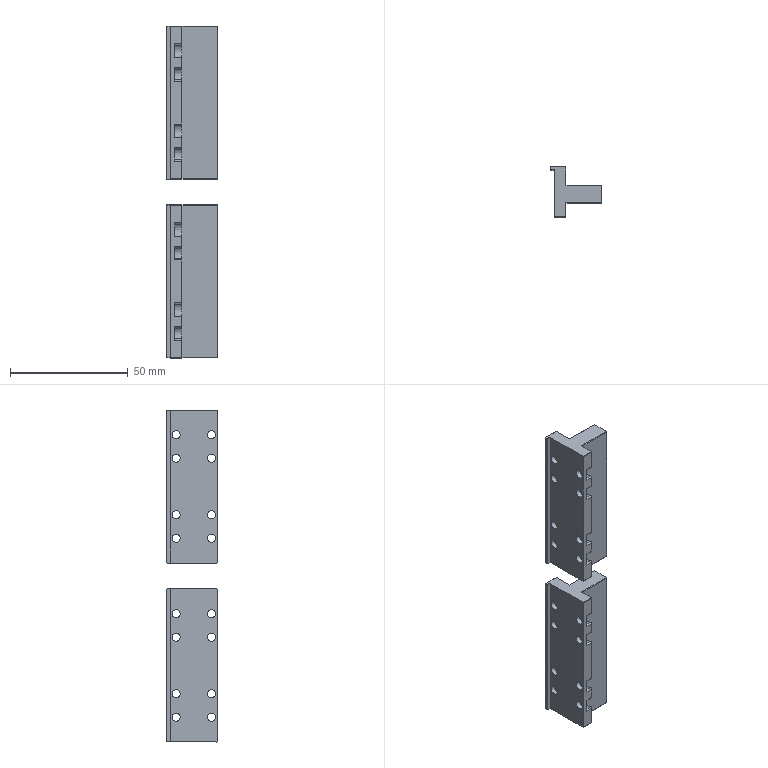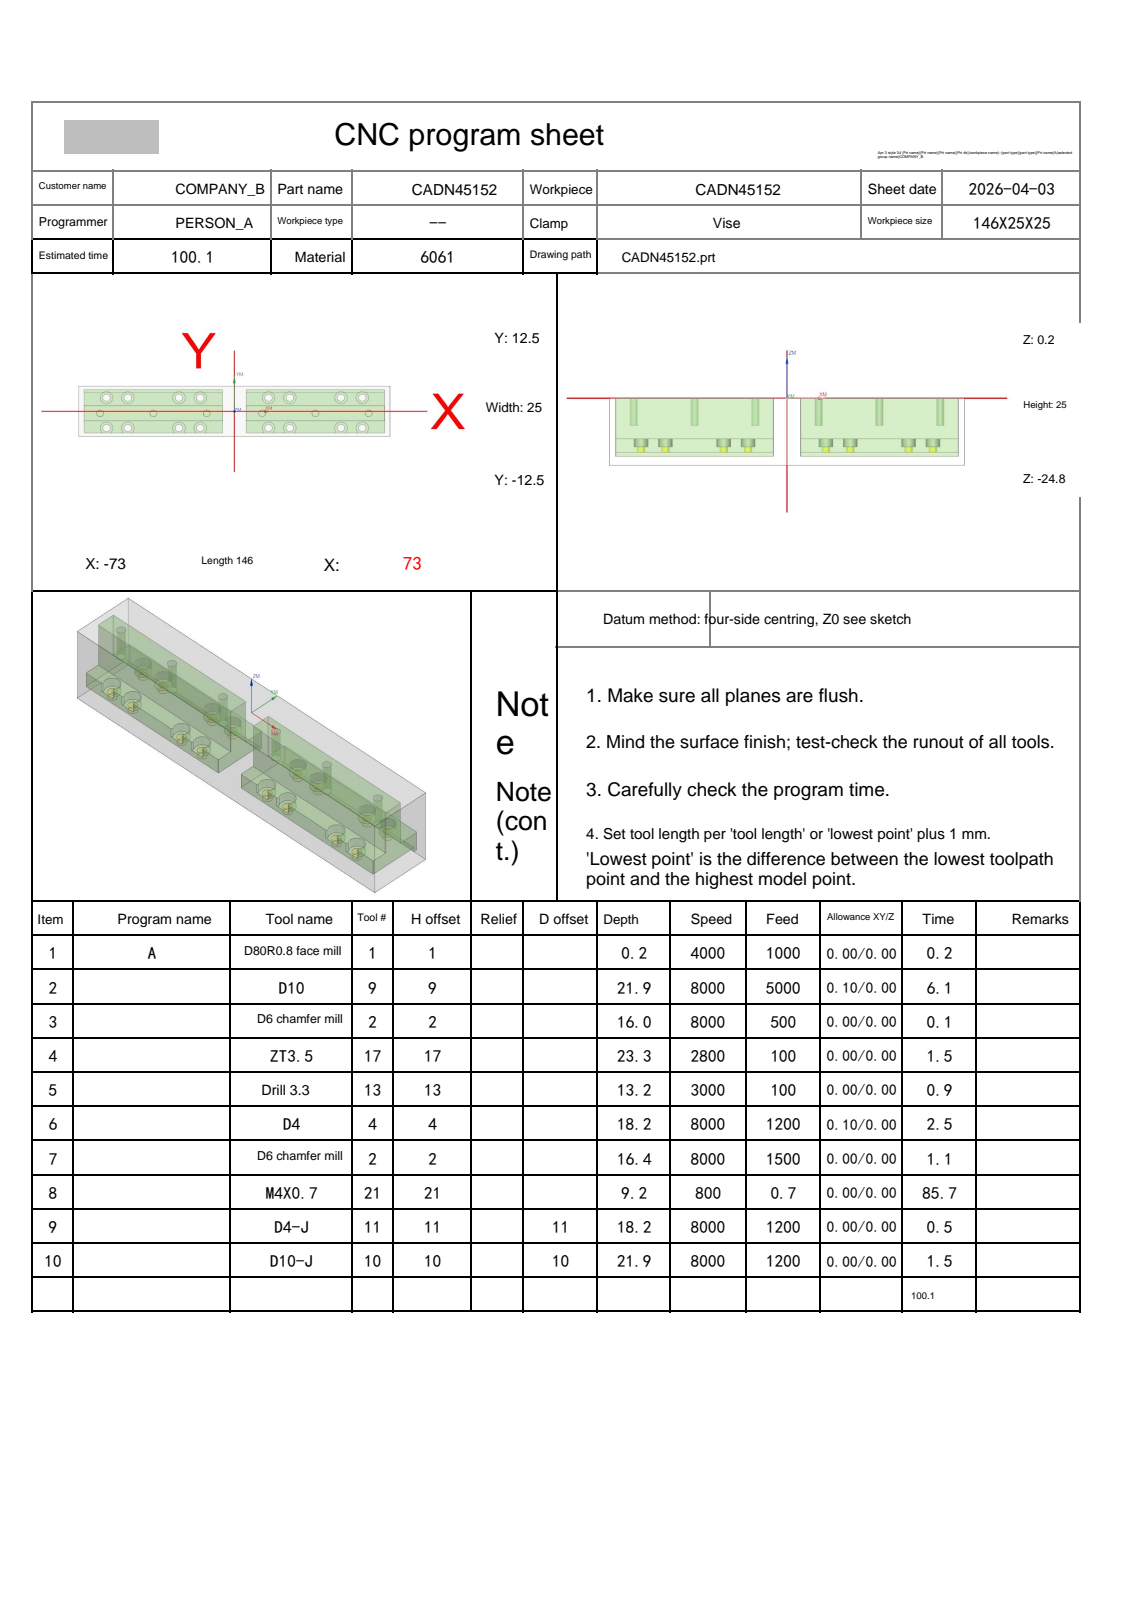NC program | NX | posted by the shop | part box 21.5 x 21.5 x 141 mm
Lines 1 to 35 of 7245:
%
O0001
(Machine time: 179.06 MIN)
(===Total Tool:9===)
(T1=D80R0.8 face mill D=80.  R=0.8  D-  H01 Z=-0.   )
(T9=D10     D=10.  R=0.   D-  H09 Z=-21.7 )
(T2=D6 chamfer mill   D=6.   R=0.   D-  H02 Z=-16.2 )
(T17=ZT3.5  D=3.5  DR_a=118 D-  H17 Z=-23.05)
(T13=drill 3.3  D=3.3  DR_a=118 D-  H13 Z=-13.  )
(T4=D4      D=4.   R=0.   D-  H04 Z=-18.  )
(T21=M4X0.7 D=3.3  DR_a=180 D-  H21 Z=-9.   )
(T11=D4-J   D=4.   R=0.   D11 H11 Z=-18.  )
(T10=D10-J  D=10.  R=0.   D10 H10 Z=-21.7 )
G80 G90 G17 G49 G40
G91 G28 Z0
M01
N1 T01 M06
(D80R0.8 face mill  D=80. R=0.8 H=01 ce=0.00 di=0.00)
G00 G90 G54 X-115.5 Y0.0 M03 S4000
G43 H01 Z20.
M08
Z2.
G01 Z0.0 F1000.
X-110.5
X110.5
X115.5
Z2.
G00 Z20.
G91 G28 Z0.0
M05
M09
G91 G28 Z0.0
M01